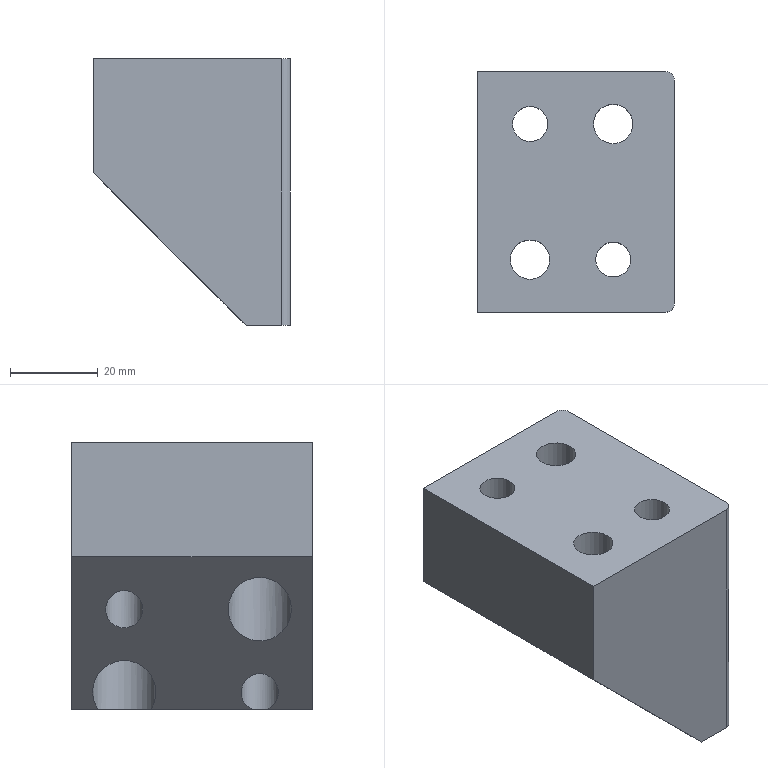Part | NX | features solid 2 | 1 solid | 21 faces | box 45 x 55 x 61 mm | volume 101618 mm3 | plane 11 | cylinder 10 | commonest cylinder face diameters 4 x2 8.001 x2 8.5 x2 9 x2 14.5 x2
STEP:
#1=CARTESIAN_POINT('',(625.792,50.391,-6.));
#2=VERTEX_POINT('',#1);
#3=CARTESIAN_POINT('',(625.792,47.079,-6.));
#4=VERTEX_POINT('',#3);
#5=CARTESIAN_POINT('',(621.878,48.735,-6.));
#6=DIRECTION('',(0.,0.,1.));
#7=DIRECTION('',(1.,0.,0.));
#8=AXIS2_PLACEMENT_3D('',#5,#6,#7);
#9=CIRCLE('',#8,4.25);
#10=EDGE_CURVE('',#2,#4,#9,.F.);
#11=ORIENTED_EDGE('',*,*,#10,.F.);
#12=CARTESIAN_POINT('',(625.792,73.632,-6.));
#13=VERTEX_POINT('',#12);
#14=CARTESIAN_POINT('',(625.792,53.735,-6.));
#15=DIRECTION('',(0.,-1.,0.));
#16=VECTOR('',#15,1000.);
#17=LINE('',#14,#16);
#18=EDGE_CURVE('',#13,#2,#17,.T.);
#19=ORIENTED_EDGE('',*,*,#18,.F.);
#20=CARTESIAN_POINT('',(625.792,85.837,-6.));
#21=VERTEX_POINT('',#20);
#22=CARTESIAN_POINT('',(621.878,79.735,-6.));
#23=DIRECTION('',(0.,0.,-1.));
#24=DIRECTION('',(1.,0.,0.));
#25=AXIS2_PLACEMENT_3D('',#22,#23,#24);
#26=CIRCLE('',#25,7.25);
#27=EDGE_CURVE('',#13,#21,#26,.F.);
#28=ORIENTED_EDGE('',*,*,#27,.T.);
#29=CARTESIAN_POINT('',(625.792,91.735,-6.));
#30=VERTEX_POINT('',#29);
#31=CARTESIAN_POINT('',(625.792,53.735,-6.));
#32=DIRECTION('',(0.,-1.,0.));
#33=VECTOR('',#32,1000.);
#34=LINE('',#31,#33);
#35=EDGE_CURVE('',#30,#21,#34,.T.);
#36=ORIENTED_EDGE('',*,*,#35,.F.);
#37=CARTESIAN_POINT('',(633.878,91.735,-6.));
#38=VERTEX_POINT('',#37);
#39=CARTESIAN_POINT('',(735.,91.735,-6.));
#40=DIRECTION('',(-1.,0.,0.));
#41=VECTOR('',#40,1000.);
#42=LINE('',#39,#41);
#43=EDGE_CURVE('',#30,#38,#42,.F.);
#44=ORIENTED_EDGE('',*,*,#43,.T.);
#45=CARTESIAN_POINT('',(635.878,89.735,-6.));
#46=VERTEX_POINT('',#45);
#47=CARTESIAN_POINT('',(633.878,89.735,-6.));
#48=DIRECTION('',(0.,0.,1.));
#49=DIRECTION('',(1.,0.,0.));
#50=AXIS2_PLACEMENT_3D('',#47,#48,#49);
#51=CIRCLE('',#50,2.);
#52=EDGE_CURVE('',#38,#46,#51,.F.);
#53=ORIENTED_EDGE('',*,*,#52,.T.);
#54=CARTESIAN_POINT('',(635.878,38.735,-6.));
#55=VERTEX_POINT('',#54);
#56=CARTESIAN_POINT('',(635.878,53.735,-6.));
#57=DIRECTION('',(0.,-1.,0.));
#58=VECTOR('',#57,1000.);
#59=LINE('',#56,#58);
#60=EDGE_CURVE('',#55,#46,#59,.F.);
#61=ORIENTED_EDGE('',*,*,#60,.F.);
#62=CARTESIAN_POINT('',(633.878,36.735,-6.));
#63=VERTEX_POINT('',#62);
#64=CARTESIAN_POINT('',(633.878,38.735,-6.));
#65=DIRECTION('',(0.,0.,1.));
#66=DIRECTION('',(1.,0.,0.));
#67=AXIS2_PLACEMENT_3D('',#64,#65,#66);
#68=CIRCLE('',#67,2.);
#69=EDGE_CURVE('',#55,#63,#68,.F.);
#70=ORIENTED_EDGE('',*,*,#69,.T.);
#71=CARTESIAN_POINT('',(625.792,36.735,-6.));
#72=VERTEX_POINT('',#71);
#73=CARTESIAN_POINT('',(585.878,36.735,-6.));
#74=DIRECTION('',(1.,0.,0.));
#75=VECTOR('',#74,1000.);
#76=LINE('',#73,#75);
#77=EDGE_CURVE('',#72,#63,#76,.T.);
#78=ORIENTED_EDGE('',*,*,#77,.F.);
#79=CARTESIAN_POINT('',(625.792,53.735,-6.));
#80=DIRECTION('',(0.,-1.,0.));
#81=VECTOR('',#80,1000.);
#82=LINE('',#79,#81);
#83=EDGE_CURVE('',#4,#72,#82,.T.);
#84=ORIENTED_EDGE('',*,*,#83,.F.);
#85=EDGE_LOOP('',(#11,#19,#28,#36,#44,#53,#61,#70,#78,#84));
#86=FACE_BOUND('',#85,.T.);
#87=CARTESIAN_POINT('',(735.,-87.419,-6.));
#88=DIRECTION('',(0.,0.,1.));
#89=DIRECTION('',(-0.9997,-0.02352,0.));
#90=AXIS2_PLACEMENT_3D('',#87,#88,#89);
#91=PLANE('',#90);
#92=ADVANCED_FACE('',(#86),#91,.F.);
#93=CARTESIAN_POINT('',(590.878,36.735,28.914));
#94=VERTEX_POINT('',#93);
#95=CARTESIAN_POINT('',(590.878,36.735,55.));
#96=VERTEX_POINT('',#95);
#97=CARTESIAN_POINT('',(590.878,36.735,-5.));
#98=DIRECTION('',(0.,0.,-1.));
#99=VECTOR('',#98,1000.);
#100=LINE('',#97,#99);
#101=EDGE_CURVE('',#94,#96,#100,.F.);
#102=ORIENTED_EDGE('',*,*,#101,.T.);
#103=CARTESIAN_POINT('',(590.878,91.735,55.));
#104=VERTEX_POINT('',#103);
#105=CARTESIAN_POINT('',(590.878,53.735,55.));
#106=DIRECTION('',(0.,1.,0.));
#107=VECTOR('',#106,1000.);
#108=LINE('',#105,#107);
#109=EDGE_CURVE('',#96,#104,#108,.T.);
#110=ORIENTED_EDGE('',*,*,#109,.T.);
#111=CARTESIAN_POINT('',(590.878,91.735,28.914));
#112=VERTEX_POINT('',#111);
#113=CARTESIAN_POINT('',(590.878,91.735,-5.));
#114=DIRECTION('',(0.,0.,-1.));
#115=VECTOR('',#114,1000.);
#116=LINE('',#113,#115);
#117=EDGE_CURVE('',#104,#112,#116,.T.);
#118=ORIENTED_EDGE('',*,*,#117,.T.);
#119=CARTESIAN_POINT('',(590.878,53.735,28.914));
#120=DIRECTION('',(0.,1.,0.));
#121=VECTOR('',#120,1000.);
#122=LINE('',#119,#121);
#123=EDGE_CURVE('',#112,#94,#122,.F.);
#124=ORIENTED_EDGE('',*,*,#123,.T.);
#125=EDGE_LOOP('',(#102,#110,#118,#124));
#126=FACE_BOUND('',#125,.T.);
#127=CARTESIAN_POINT('',(590.878,53.735,-5.));
#128=DIRECTION('',(-1.,0.,0.));
#129=DIRECTION('',(0.,0.,1.));
#130=AXIS2_PLACEMENT_3D('',#127,#128,#129);
#131=PLANE('',#130);
#132=ADVANCED_FACE('',(#126),#131,.T.);
#133=CARTESIAN_POINT('',(635.878,89.735,55.));
#134=VERTEX_POINT('',#133);
#135=CARTESIAN_POINT('',(635.878,89.735,-5.));
#136=DIRECTION('',(0.,0.,1.));
#137=VECTOR('',#136,1000.);
#138=LINE('',#135,#137);
#139=EDGE_CURVE('',#46,#134,#138,.T.);
#140=ORIENTED_EDGE('',*,*,#139,.T.);
#141=CARTESIAN_POINT('',(635.878,38.735,55.));
#142=VERTEX_POINT('',#141);
#143=CARTESIAN_POINT('',(635.878,53.735,55.));
#144=DIRECTION('',(0.,-1.,0.));
#145=VECTOR('',#144,1000.);
#146=LINE('',#143,#145);
#147=EDGE_CURVE('',#134,#142,#146,.T.);
#148=ORIENTED_EDGE('',*,*,#147,.T.);
#149=CARTESIAN_POINT('',(635.878,38.735,-5.));
#150=DIRECTION('',(0.,0.,1.));
#151=VECTOR('',#150,1000.);
#152=LINE('',#149,#151);
#153=EDGE_CURVE('',#142,#55,#152,.F.);
#154=ORIENTED_EDGE('',*,*,#153,.T.);
#155=ORIENTED_EDGE('',*,*,#60,.T.);
#156=EDGE_LOOP('',(#140,#148,#154,#155));
#157=FACE_BOUND('',#156,.T.);
#158=CARTESIAN_POINT('',(635.878,53.735,-5.));
#159=DIRECTION('',(1.,0.,0.));
#160=DIRECTION('',(0.,0.,-1.));
#161=AXIS2_PLACEMENT_3D('',#158,#159,#160);
#162=PLANE('',#161);
#163=ADVANCED_FACE('',(#157),#162,.T.);
#164=CARTESIAN_POINT('',(633.878,36.735,55.));
#165=VERTEX_POINT('',#164);
#166=CARTESIAN_POINT('',(633.878,36.735,-5.));
#167=DIRECTION('',(0.,0.,-1.));
#168=VECTOR('',#167,1000.);
#169=LINE('',#166,#168);
#170=EDGE_CURVE('',#63,#165,#169,.F.);
#171=ORIENTED_EDGE('',*,*,#170,.T.);
#172=CARTESIAN_POINT('',(585.878,36.735,55.));
#173=DIRECTION('',(1.,0.,0.));
#174=VECTOR('',#173,1000.);
#175=LINE('',#172,#174);
#176=EDGE_CURVE('',#165,#96,#175,.F.);
#177=ORIENTED_EDGE('',*,*,#176,.T.);
#178=ORIENTED_EDGE('',*,*,#101,.F.);
#179=CARTESIAN_POINT('',(605.335,36.735,14.457));
#180=DIRECTION('',(0.7071,0.,-0.7071));
#181=VECTOR('',#180,1000.);
#182=LINE('',#179,#181);
#183=EDGE_CURVE('',#94,#72,#182,.T.);
#184=ORIENTED_EDGE('',*,*,#183,.T.);
#185=ORIENTED_EDGE('',*,*,#77,.T.);
#186=EDGE_LOOP('',(#171,#177,#178,#184,#185));
#187=FACE_BOUND('',#186,.T.);
#188=CARTESIAN_POINT('',(585.878,36.735,-5.));
#189=DIRECTION('',(0.,1.,0.));
#190=DIRECTION('',(0.,0.,1.));
#191=AXIS2_PLACEMENT_3D('',#188,#189,#190);
#192=PLANE('',#191);
#193=ADVANCED_FACE('',(#187),#192,.F.);
#194=ORIENTED_EDGE('',*,*,#153,.F.);
#195=CARTESIAN_POINT('',(633.878,38.735,55.));
#196=DIRECTION('',(0.,0.,1.));
#197=DIRECTION('',(1.,0.,0.));
#198=AXIS2_PLACEMENT_3D('',#195,#196,#197);
#199=CIRCLE('',#198,2.);
#200=EDGE_CURVE('',#142,#165,#199,.F.);
#201=ORIENTED_EDGE('',*,*,#200,.T.);
#202=ORIENTED_EDGE('',*,*,#170,.F.);
#203=ORIENTED_EDGE('',*,*,#69,.F.);
#204=EDGE_LOOP('',(#194,#201,#202,#203));
#205=FACE_BOUND('',#204,.T.);
#206=CARTESIAN_POINT('',(633.878,38.735,-5.));
#207=DIRECTION('',(0.,0.,1.));
#208=DIRECTION('',(1.,0.,0.));
#209=AXIS2_PLACEMENT_3D('',#206,#207,#208);
#210=CYLINDRICAL_SURFACE('',#209,2.);
#211=ADVANCED_FACE('',(#205),#210,.T.);
#212=ORIENTED_EDGE('',*,*,#117,.F.);
#213=CARTESIAN_POINT('',(633.878,91.735,55.));
#214=VERTEX_POINT('',#213);
#215=CARTESIAN_POINT('',(619.878,91.735,55.));
#216=DIRECTION('',(1.,0.,0.));
#217=VECTOR('',#216,1000.);
#218=LINE('',#215,#217);
#219=EDGE_CURVE('',#104,#214,#218,.T.);
#220=ORIENTED_EDGE('',*,*,#219,.T.);
#221=CARTESIAN_POINT('',(633.878,91.735,22.));
#222=DIRECTION('',(0.,0.,1.));
#223=VECTOR('',#222,1000.);
#224=LINE('',#221,#223);
#225=EDGE_CURVE('',#214,#38,#224,.F.);
#226=ORIENTED_EDGE('',*,*,#225,.T.);
#227=ORIENTED_EDGE('',*,*,#43,.F.);
#228=CARTESIAN_POINT('',(616.585,91.735,3.207));
#229=DIRECTION('',(-0.7071,0.,0.7071));
#230=VECTOR('',#229,1000.);
#231=LINE('',#228,#230);
#232=EDGE_CURVE('',#112,#30,#231,.F.);
#233=ORIENTED_EDGE('',*,*,#232,.F.);
#234=EDGE_LOOP('',(#212,#220,#226,#227,#233));
#235=FACE_BOUND('',#234,.T.);
#236=CARTESIAN_POINT('',(619.878,91.735,22.));
#237=DIRECTION('',(0.,1.,0.));
#238=DIRECTION('',(0.,0.,1.));
#239=AXIS2_PLACEMENT_3D('',#236,#237,#238);
#240=PLANE('',#239);
#241=ADVANCED_FACE('',(#235),#240,.T.);
#242=ORIENTED_EDGE('',*,*,#225,.F.);
#243=CARTESIAN_POINT('',(633.878,89.735,55.));
#244=DIRECTION('',(0.,0.,1.));
#245=DIRECTION('',(1.,0.,0.));
#246=AXIS2_PLACEMENT_3D('',#243,#244,#245);
#247=CIRCLE('',#246,2.);
#248=EDGE_CURVE('',#214,#134,#247,.F.);
#249=ORIENTED_EDGE('',*,*,#248,.T.);
#250=ORIENTED_EDGE('',*,*,#139,.F.);
#251=ORIENTED_EDGE('',*,*,#52,.F.);
#252=EDGE_LOOP('',(#242,#249,#250,#251));
#253=FACE_BOUND('',#252,.T.);
#254=CARTESIAN_POINT('',(633.878,89.735,-5.));
#255=DIRECTION('',(0.,0.,1.));
#256=DIRECTION('',(1.,0.,0.));
#257=AXIS2_PLACEMENT_3D('',#254,#255,#256);
#258=CYLINDRICAL_SURFACE('',#257,2.);
#259=ADVANCED_FACE('',(#253),#258,.T.);
#260=CARTESIAN_POINT('',(621.878,48.735,-2.086));
#261=DIRECTION('',(0.7071,0.,0.7071));
#262=DIRECTION('',(-0.7071,0.,0.7071));
#263=AXIS2_PLACEMENT_3D('',#260,#261,#262);
#264=ELLIPSE('',#263,6.01,4.25);
#265=EDGE_CURVE('',#4,#2,#264,.F.);
#266=ORIENTED_EDGE('',*,*,#265,.F.);
#267=ORIENTED_EDGE('',*,*,#83,.T.);
#268=ORIENTED_EDGE('',*,*,#183,.F.);
#269=ORIENTED_EDGE('',*,*,#123,.F.);
#270=ORIENTED_EDGE('',*,*,#232,.T.);
#271=ORIENTED_EDGE('',*,*,#35,.T.);
#272=CARTESIAN_POINT('',(621.878,79.735,-2.086));
#273=DIRECTION('',(0.7071,0.,0.7071));
#274=DIRECTION('',(-0.7071,0.,0.7071));
#275=AXIS2_PLACEMENT_3D('',#272,#273,#274);
#276=ELLIPSE('',#275,10.253,7.25);
#277=EDGE_CURVE('',#13,#21,#276,.F.);
#278=ORIENTED_EDGE('',*,*,#277,.F.);
#279=ORIENTED_EDGE('',*,*,#18,.T.);
#280=EDGE_LOOP('',(#266,#267,#268,#269,#270,#271,#278,#279));
#281=FACE_BOUND('',#280,.T.);
#282=CARTESIAN_POINT('',(598.628,79.735,21.164));
#283=VERTEX_POINT('',#282);
#284=CARTESIAN_POINT('',(602.878,79.735,16.914));
#285=DIRECTION('',(0.7071,0.,0.7071));
#286=DIRECTION('',(-0.7071,0.,0.7071));
#287=AXIS2_PLACEMENT_3D('',#284,#285,#286);
#288=ELLIPSE('',#287,6.01,4.25);
#289=EDGE_CURVE('',#283,#283,#288,.F.);
#290=ORIENTED_EDGE('',*,*,#289,.F.);
#291=EDGE_LOOP('',(#290));
#292=FACE_BOUND('',#291,.T.);
#293=CARTESIAN_POINT('',(595.628,48.735,24.164));
#294=VERTEX_POINT('',#293);
#295=CARTESIAN_POINT('',(602.878,48.735,16.914));
#296=DIRECTION('',(0.7071,0.,0.7071));
#297=DIRECTION('',(-0.7071,0.,0.7071));
#298=AXIS2_PLACEMENT_3D('',#295,#296,#297);
#299=ELLIPSE('',#298,10.253,7.25);
#300=EDGE_CURVE('',#294,#294,#299,.F.);
#301=ORIENTED_EDGE('',*,*,#300,.F.);
#302=EDGE_LOOP('',(#301));
#303=FACE_BOUND('',#302,.T.);
#304=CARTESIAN_POINT('',(616.585,53.735,3.207));
#305=DIRECTION('',(0.7071,0.,0.7071));
#306=DIRECTION('',(0.,-1.,0.));
#307=AXIS2_PLACEMENT_3D('',#304,#305,#306);
#308=PLANE('',#307);
#309=ADVANCED_FACE('',(#281,#292,#303),#308,.F.);
#310=CARTESIAN_POINT('',(625.878,48.735,55.));
#311=VERTEX_POINT('',#310);
#312=CARTESIAN_POINT('',(621.878,48.735,55.));
#313=DIRECTION('',(0.,0.,1.));
#314=DIRECTION('',(1.,0.,0.));
#315=AXIS2_PLACEMENT_3D('',#312,#313,#314);
#316=CIRCLE('',#315,4.);
#317=EDGE_CURVE('',#311,#311,#316,.T.);
#318=ORIENTED_EDGE('',*,*,#317,.F.);
#319=EDGE_LOOP('',(#318));
#320=FACE_BOUND('',#319,.T.);
#321=CARTESIAN_POINT('',(606.878,79.735,55.));
#322=VERTEX_POINT('',#321);
#323=CARTESIAN_POINT('',(602.878,79.735,55.));
#324=DIRECTION('',(0.,0.,1.));
#325=DIRECTION('',(1.,0.,0.));
#326=AXIS2_PLACEMENT_3D('',#323,#324,#325);
#327=CIRCLE('',#326,4.);
#328=EDGE_CURVE('',#322,#322,#327,.T.);
#329=ORIENTED_EDGE('',*,*,#328,.F.);
#330=EDGE_LOOP('',(#329));
#331=FACE_BOUND('',#330,.T.);
#332=CARTESIAN_POINT('',(626.378,79.735,55.));
#333=VERTEX_POINT('',#332);
#334=CARTESIAN_POINT('',(621.878,79.735,55.));
#335=DIRECTION('',(0.,0.,1.));
#336=DIRECTION('',(1.,0.,0.));
#337=AXIS2_PLACEMENT_3D('',#334,#335,#336);
#338=CIRCLE('',#337,4.5);
#339=EDGE_CURVE('',#333,#333,#338,.T.);
#340=ORIENTED_EDGE('',*,*,#339,.F.);
#341=EDGE_LOOP('',(#340));
#342=FACE_BOUND('',#341,.T.);
#343=CARTESIAN_POINT('',(607.378,48.735,55.));
#344=VERTEX_POINT('',#343);
#345=CARTESIAN_POINT('',(602.878,48.735,55.));
#346=DIRECTION('',(0.,0.,1.));
#347=DIRECTION('',(1.,0.,0.));
#348=AXIS2_PLACEMENT_3D('',#345,#346,#347);
#349=CIRCLE('',#348,4.5);
#350=EDGE_CURVE('',#344,#344,#349,.T.);
#351=ORIENTED_EDGE('',*,*,#350,.F.);
#352=EDGE_LOOP('',(#351));
#353=FACE_BOUND('',#352,.T.);
#354=ORIENTED_EDGE('',*,*,#176,.F.);
#355=ORIENTED_EDGE('',*,*,#200,.F.);
#356=ORIENTED_EDGE('',*,*,#147,.F.);
#357=ORIENTED_EDGE('',*,*,#248,.F.);
#358=ORIENTED_EDGE('',*,*,#219,.F.);
#359=ORIENTED_EDGE('',*,*,#109,.F.);
#360=EDGE_LOOP('',(#354,#355,#356,#357,#358,#359));
#361=FACE_BOUND('',#360,.T.);
#362=CARTESIAN_POINT('',(612.,0.,55.));
#363=DIRECTION('',(0.,0.,1.));
#364=DIRECTION('',(1.,0.,0.));
#365=AXIS2_PLACEMENT_3D('',#362,#363,#364);
#366=PLANE('',#365);
#367=ADVANCED_FACE('',(#320,#331,#342,#353,#361),#366,.T.);
#368=ORIENTED_EDGE('',*,*,#350,.T.);
#369=EDGE_LOOP('',(#368));
#370=FACE_BOUND('',#369,.T.);
#371=CARTESIAN_POINT('',(598.378,48.735,30.));
#372=VERTEX_POINT('',#371);
#373=CARTESIAN_POINT('',(602.878,48.735,30.));
#374=DIRECTION('',(0.,0.,-1.));
#375=DIRECTION('',(-1.,0.,0.));
#376=AXIS2_PLACEMENT_3D('',#373,#374,#375);
#377=CIRCLE('',#376,4.5);
#378=EDGE_CURVE('',#372,#372,#377,.F.);
#379=ORIENTED_EDGE('',*,*,#378,.F.);
#380=EDGE_LOOP('',(#379));
#381=FACE_BOUND('',#380,.T.);
#382=CARTESIAN_POINT('',(602.878,48.735,-8.));
#383=DIRECTION('',(0.,0.,1.));
#384=DIRECTION('',(1.,0.,0.));
#385=AXIS2_PLACEMENT_3D('',#382,#383,#384);
#386=CYLINDRICAL_SURFACE('',#385,4.5);
#387=ADVANCED_FACE('',(#370,#381),#386,.F.);
#388=ORIENTED_EDGE('',*,*,#378,.T.);
#389=EDGE_LOOP('',(#388));
#390=FACE_BOUND('',#389,.T.);
#391=CARTESIAN_POINT('',(610.128,48.735,30.));
#392=VERTEX_POINT('',#391);
#393=CARTESIAN_POINT('',(602.878,48.735,30.));
#394=DIRECTION('',(0.,0.,1.));
#395=DIRECTION('',(1.,0.,0.));
#396=AXIS2_PLACEMENT_3D('',#393,#394,#395);
#397=CIRCLE('',#396,7.25);
#398=EDGE_CURVE('',#392,#392,#397,.T.);
#399=ORIENTED_EDGE('',*,*,#398,.F.);
#400=EDGE_LOOP('',(#399));
#401=FACE_BOUND('',#400,.T.);
#402=CARTESIAN_POINT('',(602.878,48.735,30.));
#403=DIRECTION('',(0.,0.,1.));
#404=DIRECTION('',(-1.,0.,0.));
#405=AXIS2_PLACEMENT_3D('',#402,#403,#404);
#406=PLANE('',#405);
#407=ADVANCED_FACE('',(#390,#401),#406,.F.);
#408=ORIENTED_EDGE('',*,*,#300,.T.);
#409=EDGE_LOOP('',(#408));
#410=FACE_BOUND('',#409,.T.);
#411=ORIENTED_EDGE('',*,*,#398,.T.);
#412=EDGE_LOOP('',(#411));
#413=FACE_BOUND('',#412,.T.);
#414=CARTESIAN_POINT('',(602.878,48.735,-6.));
#415=DIRECTION('',(0.,0.,1.));
#416=DIRECTION('',(1.,0.,0.));
#417=AXIS2_PLACEMENT_3D('',#414,#415,#416);
#418=CYLINDRICAL_SURFACE('',#417,7.25);
#419=ADVANCED_FACE('',(#410,#413),#418,.F.);
#420=ORIENTED_EDGE('',*,*,#339,.T.);
#421=EDGE_LOOP('',(#420));
#422=FACE_BOUND('',#421,.T.);
#423=CARTESIAN_POINT('',(617.378,79.735,30.));
#424=VERTEX_POINT('',#423);
#425=CARTESIAN_POINT('',(621.878,79.735,30.));
#426=DIRECTION('',(0.,0.,-1.));
#427=DIRECTION('',(-1.,0.,0.));
#428=AXIS2_PLACEMENT_3D('',#425,#426,#427);
#429=CIRCLE('',#428,4.5);
#430=EDGE_CURVE('',#424,#424,#429,.F.);
#431=ORIENTED_EDGE('',*,*,#430,.F.);
#432=EDGE_LOOP('',(#431));
#433=FACE_BOUND('',#432,.T.);
#434=CARTESIAN_POINT('',(621.878,79.735,-8.));
#435=DIRECTION('',(0.,0.,1.));
#436=DIRECTION('',(1.,0.,0.));
#437=AXIS2_PLACEMENT_3D('',#434,#435,#436);
#438=CYLINDRICAL_SURFACE('',#437,4.5);
#439=ADVANCED_FACE('',(#422,#433),#438,.F.);
#440=ORIENTED_EDGE('',*,*,#430,.T.);
#441=EDGE_LOOP('',(#440));
#442=FACE_BOUND('',#441,.T.);
#443=CARTESIAN_POINT('',(629.128,79.735,30.));
#444=VERTEX_POINT('',#443);
#445=CARTESIAN_POINT('',(621.878,79.735,30.));
#446=DIRECTION('',(0.,0.,1.));
#447=DIRECTION('',(1.,0.,0.));
#448=AXIS2_PLACEMENT_3D('',#445,#446,#447);
#449=CIRCLE('',#448,7.25);
#450=EDGE_CURVE('',#444,#444,#449,.T.);
#451=ORIENTED_EDGE('',*,*,#450,.F.);
#452=EDGE_LOOP('',(#451));
#453=FACE_BOUND('',#452,.T.);
#454=CARTESIAN_POINT('',(621.878,79.735,30.));
#455=DIRECTION('',(0.,0.,1.));
#456=DIRECTION('',(-1.,0.,0.));
#457=AXIS2_PLACEMENT_3D('',#454,#455,#456);
#458=PLANE('',#457);
#459=ADVANCED_FACE('',(#442,#453),#458,.F.);
#460=ORIENTED_EDGE('',*,*,#277,.T.);
#461=ORIENTED_EDGE('',*,*,#27,.F.);
#462=EDGE_LOOP('',(#460,#461));
#463=FACE_BOUND('',#462,.T.);
#464=ORIENTED_EDGE('',*,*,#450,.T.);
#465=EDGE_LOOP('',(#464));
#466=FACE_BOUND('',#465,.T.);
#467=CARTESIAN_POINT('',(621.878,79.735,-6.));
#468=DIRECTION('',(0.,0.,1.));
#469=DIRECTION('',(1.,0.,0.));
#470=AXIS2_PLACEMENT_3D('',#467,#468,#469);
#471=CYLINDRICAL_SURFACE('',#470,7.25);
#472=ADVANCED_FACE('',(#463,#466),#471,.F.);
#473=ORIENTED_EDGE('',*,*,#328,.T.);
#474=EDGE_LOOP('',(#473));
#475=FACE_BOUND('',#474,.T.);
#476=CARTESIAN_POINT('',(598.877,79.735,34.));
#477=VERTEX_POINT('',#476);
#478=CARTESIAN_POINT('',(602.878,79.735,34.));
#479=DIRECTION('',(0.,0.,-1.));
#480=DIRECTION('',(-1.,0.,0.));
#481=AXIS2_PLACEMENT_3D('',#478,#479,#480);
#482=CIRCLE('',#481,4.);
#483=EDGE_CURVE('',#477,#477,#482,.F.);
#484=ORIENTED_EDGE('',*,*,#483,.F.);
#485=EDGE_LOOP('',(#484));
#486=FACE_BOUND('',#485,.T.);
#487=CARTESIAN_POINT('',(602.878,79.735,-8.));
#488=DIRECTION('',(0.,0.,1.));
#489=DIRECTION('',(1.,0.,0.));
#490=AXIS2_PLACEMENT_3D('',#487,#488,#489);
#491=CYLINDRICAL_SURFACE('',#490,4.);
#492=ADVANCED_FACE('',(#475,#486),#491,.F.);
#493=ORIENTED_EDGE('',*,*,#483,.T.);
#494=EDGE_LOOP('',(#493));
#495=FACE_BOUND('',#494,.T.);
#496=CARTESIAN_POINT('',(607.128,79.735,34.));
#497=VERTEX_POINT('',#496);
#498=CARTESIAN_POINT('',(602.878,79.735,34.));
#499=DIRECTION('',(0.,0.,1.));
#500=DIRECTION('',(1.,0.,0.));
#501=AXIS2_PLACEMENT_3D('',#498,#499,#500);
#502=CIRCLE('',#501,4.25);
#503=EDGE_CURVE('',#497,#497,#502,.T.);
#504=ORIENTED_EDGE('',*,*,#503,.F.);
#505=EDGE_LOOP('',(#504));
#506=FACE_BOUND('',#505,.T.);
#507=CARTESIAN_POINT('',(602.878,79.735,34.));
#508=DIRECTION('',(0.,0.,1.));
#509=DIRECTION('',(-1.,0.,0.));
#510=AXIS2_PLACEMENT_3D('',#507,#508,#509);
#511=PLANE('',#510);
#512=ADVANCED_FACE('',(#495,#506),#511,.F.);
#513=ORIENTED_EDGE('',*,*,#289,.T.);
#514=EDGE_LOOP('',(#513));
#515=FACE_BOUND('',#514,.T.);
#516=ORIENTED_EDGE('',*,*,#503,.T.);
#517=EDGE_LOOP('',(#516));
#518=FACE_BOUND('',#517,.T.);
#519=CARTESIAN_POINT('',(602.878,79.735,-8.));
#520=DIRECTION('',(0.,0.,1.));
#521=DIRECTION('',(1.,0.,0.));
#522=AXIS2_PLACEMENT_3D('',#519,#520,#521);
#523=CYLINDRICAL_SURFACE('',#522,4.25);
#524=ADVANCED_FACE('',(#515,#518),#523,.F.);
#525=ORIENTED_EDGE('',*,*,#317,.T.);
#526=EDGE_LOOP('',(#525));
#527=FACE_BOUND('',#526,.T.);
#528=CARTESIAN_POINT('',(617.877,48.735,34.));
#529=VERTEX_POINT('',#528);
#530=CARTESIAN_POINT('',(621.878,48.735,34.));
#531=DIRECTION('',(0.,0.,-1.));
#532=DIRECTION('',(-1.,0.,0.));
#533=AXIS2_PLACEMENT_3D('',#530,#531,#532);
#534=CIRCLE('',#533,4.);
#535=EDGE_CURVE('',#529,#529,#534,.F.);
#536=ORIENTED_EDGE('',*,*,#535,.F.);
#537=EDGE_LOOP('',(#536));
#538=FACE_BOUND('',#537,.T.);
#539=CARTESIAN_POINT('',(621.878,48.735,-8.));
#540=DIRECTION('',(0.,0.,1.));
#541=DIRECTION('',(1.,0.,0.));
#542=AXIS2_PLACEMENT_3D('',#539,#540,#541);
#543=CYLINDRICAL_SURFACE('',#542,4.);
#544=ADVANCED_FACE('',(#527,#538),#543,.F.);
#545=ORIENTED_EDGE('',*,*,#535,.T.);
#546=EDGE_LOOP('',(#545));
#547=FACE_BOUND('',#546,.T.);
#548=CARTESIAN_POINT('',(626.128,48.735,34.));
#549=VERTEX_POINT('',#548);
#550=CARTESIAN_POINT('',(621.878,48.735,34.));
#551=DIRECTION('',(0.,0.,1.));
#552=DIRECTION('',(1.,0.,0.));
#553=AXIS2_PLACEMENT_3D('',#550,#551,#552);
#554=CIRCLE('',#553,4.25);
#555=EDGE_CURVE('',#549,#549,#554,.T.);
#556=ORIENTED_EDGE('',*,*,#555,.F.);
#557=EDGE_LOOP('',(#556));
#558=FACE_BOUND('',#557,.T.);
#559=CARTESIAN_POINT('',(621.878,48.735,34.));
#560=DIRECTION('',(0.,0.,1.));
#561=DIRECTION('',(-1.,0.,0.));
#562=AXIS2_PLACEMENT_3D('',#559,#560,#561);
#563=PLANE('',#562);
#564=ADVANCED_FACE('',(#547,#558),#563,.F.);
#565=ORIENTED_EDGE('',*,*,#10,.T.);
#566=ORIENTED_EDGE('',*,*,#265,.T.);
#567=EDGE_LOOP('',(#565,#566));
#568=FACE_BOUND('',#567,.T.);
#569=ORIENTED_EDGE('',*,*,#555,.T.);
#570=EDGE_LOOP('',(#569));
#571=FACE_BOUND('',#570,.T.);
#572=CARTESIAN_POINT('',(621.878,48.735,-8.));
#573=DIRECTION('',(0.,0.,1.));
#574=DIRECTION('',(1.,0.,0.));
#575=AXIS2_PLACEMENT_3D('',#572,#573,#574);
#576=CYLINDRICAL_SURFACE('',#575,4.25);
#577=ADVANCED_FACE('',(#568,#571),#576,.F.);
#578=CLOSED_SHELL('',(#92,#132,#163,#193,#211,#241,#259,#309,#367,#387,#407,#419,#439,#459,#472,#492,#512,#524,#544,#564,#577));
#579=MANIFOLD_SOLID_BREP('',#578);
#580=(LENGTH_UNIT()NAMED_UNIT(*)SI_UNIT(.MILLI.,.METRE.));
#581=UNCERTAINTY_MEASURE_WITH_UNIT(LENGTH_MEASURE(0.00001),#580,'','');
#582=(NAMED_UNIT(*)PLANE_ANGLE_UNIT()SI_UNIT($,.RADIAN.));
#583=(NAMED_UNIT(*)SI_UNIT($,.STERADIAN.)SOLID_ANGLE_UNIT());
#584=(GEOMETRIC_REPRESENTATION_CONTEXT(3)GLOBAL_UNCERTAINTY_ASSIGNED_CONTEXT((#581))GLOBAL_UNIT_ASSIGNED_CONTEXT((#580,#582,#583))REPRESENTATION_CONTEXT('',''));
#585=ADVANCED_BREP_SHAPE_REPRESENTATION('',(#579),#584);